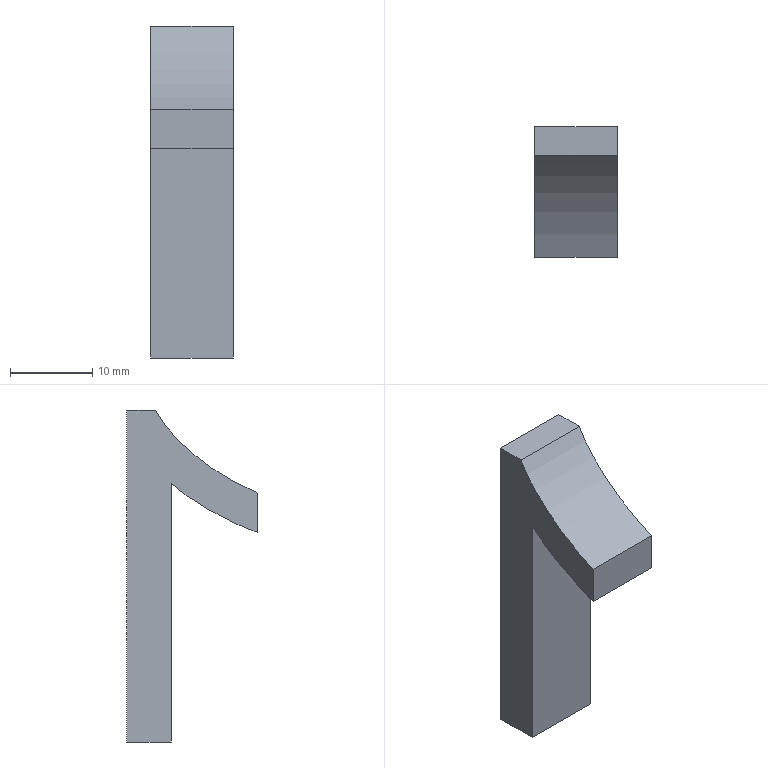Part | NX | features solid 2 | 1 solid | 9 faces | box 10 x 15.893 x 40.382 mm | volume 2722 mm3 | plane 7 | spline 2
STEP:
#1=CARTESIAN_POINT('',(2250.,-427.707,-549.618));
#2=VERTEX_POINT('',#1);
#3=CARTESIAN_POINT('',(2250.,-427.707,-590.));
#4=VERTEX_POINT('',#3);
#5=CARTESIAN_POINT('',(2250.,-427.707,-549.618));
#6=CARTESIAN_POINT('',(2250.,-427.707,-563.078));
#7=CARTESIAN_POINT('',(2250.,-427.707,-576.539));
#8=CARTESIAN_POINT('',(2250.,-427.707,-590.));
#9=B_SPLINE_CURVE_WITH_KNOTS('',3,(#5,#6,#7,#8),.UNSPECIFIED.,.F.,.F.,(4,4),(0.,0.3484),.PIECEWISE_BEZIER_KNOTS.);
#10=EDGE_CURVE('',#2,#4,#9,.T.);
#11=ORIENTED_EDGE('',*,*,#10,.F.);
#12=CARTESIAN_POINT('',(2260.,-427.707,-549.618));
#13=VERTEX_POINT('',#12);
#14=CARTESIAN_POINT('',(2260.,-427.707,-549.618));
#15=DIRECTION('',(-1.,0.,0.));
#16=VECTOR('',#15,1000.);
#17=LINE('',#14,#16);
#18=EDGE_CURVE('',#13,#2,#17,.T.);
#19=ORIENTED_EDGE('',*,*,#18,.F.);
#20=CARTESIAN_POINT('',(2260.,-427.707,-590.));
#21=VERTEX_POINT('',#20);
#22=CARTESIAN_POINT('',(2260.,-427.707,-549.618));
#23=CARTESIAN_POINT('',(2260.,-427.707,-563.078));
#24=CARTESIAN_POINT('',(2260.,-427.707,-576.539));
#25=CARTESIAN_POINT('',(2260.,-427.707,-590.));
#26=B_SPLINE_CURVE_WITH_KNOTS('',3,(#22,#23,#24,#25),.UNSPECIFIED.,.F.,.F.,(4,4),(0.,0.3484),.PIECEWISE_BEZIER_KNOTS.);
#27=EDGE_CURVE('',#13,#21,#26,.T.);
#28=ORIENTED_EDGE('',*,*,#27,.T.);
#29=CARTESIAN_POINT('',(2260.,-427.707,-590.));
#30=DIRECTION('',(-1.,0.,0.));
#31=VECTOR('',#30,1000.);
#32=LINE('',#29,#31);
#33=EDGE_CURVE('',#21,#4,#32,.T.);
#34=ORIENTED_EDGE('',*,*,#33,.T.);
#35=EDGE_LOOP('',(#11,#19,#28,#34));
#36=FACE_BOUND('',#35,.T.);
#37=CARTESIAN_POINT('',(2260.,-427.707,-549.618));
#38=DIRECTION('',(0.,1.,0.));
#39=DIRECTION('',(-1.,0.,0.));
#40=AXIS2_PLACEMENT_3D('',#37,#38,#39);
#41=PLANE('',#40);
#42=ADVANCED_FACE('',(#36),#41,.T.);
#43=CARTESIAN_POINT('',(2250.,-433.137,-590.));
#44=VERTEX_POINT('',#43);
#45=CARTESIAN_POINT('',(2250.,-427.707,-590.));
#46=CARTESIAN_POINT('',(2250.,-429.517,-590.));
#47=CARTESIAN_POINT('',(2250.,-431.327,-590.));
#48=CARTESIAN_POINT('',(2250.,-433.137,-590.));
#49=B_SPLINE_CURVE_WITH_KNOTS('',3,(#45,#46,#47,#48),.UNSPECIFIED.,.F.,.F.,(4,4),(0.3484,0.3952),.PIECEWISE_BEZIER_KNOTS.);
#50=EDGE_CURVE('',#4,#44,#49,.T.);
#51=ORIENTED_EDGE('',*,*,#50,.F.);
#52=ORIENTED_EDGE('',*,*,#33,.F.);
#53=CARTESIAN_POINT('',(2260.,-433.137,-590.));
#54=VERTEX_POINT('',#53);
#55=CARTESIAN_POINT('',(2260.,-427.707,-590.));
#56=CARTESIAN_POINT('',(2260.,-429.517,-590.));
#57=CARTESIAN_POINT('',(2260.,-431.327,-590.));
#58=CARTESIAN_POINT('',(2260.,-433.137,-590.));
#59=B_SPLINE_CURVE_WITH_KNOTS('',3,(#55,#56,#57,#58),.UNSPECIFIED.,.F.,.F.,(4,4),(0.3484,0.3952),.PIECEWISE_BEZIER_KNOTS.);
#60=EDGE_CURVE('',#21,#54,#59,.T.);
#61=ORIENTED_EDGE('',*,*,#60,.T.);
#62=CARTESIAN_POINT('',(2260.,-433.137,-590.));
#63=DIRECTION('',(-1.,0.,0.));
#64=VECTOR('',#63,1000.);
#65=LINE('',#62,#64);
#66=EDGE_CURVE('',#54,#44,#65,.T.);
#67=ORIENTED_EDGE('',*,*,#66,.T.);
#68=EDGE_LOOP('',(#51,#52,#61,#67));
#69=FACE_BOUND('',#68,.T.);
#70=CARTESIAN_POINT('',(2260.,-427.707,-590.));
#71=DIRECTION('',(0.,0.,-1.));
#72=DIRECTION('',(-1.,0.,0.));
#73=AXIS2_PLACEMENT_3D('',#70,#71,#72);
#74=PLANE('',#73);
#75=ADVANCED_FACE('',(#69),#74,.T.);
#76=CARTESIAN_POINT('',(2250.,-433.137,-558.551));
#77=VERTEX_POINT('',#76);
#78=CARTESIAN_POINT('',(2250.,-433.137,-590.));
#79=CARTESIAN_POINT('',(2250.,-433.137,-579.517));
#80=CARTESIAN_POINT('',(2250.,-433.137,-569.034));
#81=CARTESIAN_POINT('',(2250.,-433.137,-558.551));
#82=B_SPLINE_CURVE_WITH_KNOTS('',3,(#78,#79,#80,#81),.UNSPECIFIED.,.F.,.F.,(4,4),(0.3952,0.6666),.PIECEWISE_BEZIER_KNOTS.);
#83=EDGE_CURVE('',#44,#77,#82,.T.);
#84=ORIENTED_EDGE('',*,*,#83,.F.);
#85=ORIENTED_EDGE('',*,*,#66,.F.);
#86=CARTESIAN_POINT('',(2260.,-433.137,-558.551));
#87=VERTEX_POINT('',#86);
#88=CARTESIAN_POINT('',(2260.,-433.137,-590.));
#89=CARTESIAN_POINT('',(2260.,-433.137,-579.517));
#90=CARTESIAN_POINT('',(2260.,-433.137,-569.034));
#91=CARTESIAN_POINT('',(2260.,-433.137,-558.551));
#92=B_SPLINE_CURVE_WITH_KNOTS('',3,(#88,#89,#90,#91),.UNSPECIFIED.,.F.,.F.,(4,4),(0.3952,0.6666),.PIECEWISE_BEZIER_KNOTS.);
#93=EDGE_CURVE('',#54,#87,#92,.T.);
#94=ORIENTED_EDGE('',*,*,#93,.T.);
#95=CARTESIAN_POINT('',(2260.,-433.137,-558.551));
#96=DIRECTION('',(-1.,0.,0.));
#97=VECTOR('',#96,1000.);
#98=LINE('',#95,#97);
#99=EDGE_CURVE('',#87,#77,#98,.T.);
#100=ORIENTED_EDGE('',*,*,#99,.T.);
#101=EDGE_LOOP('',(#84,#85,#94,#100));
#102=FACE_BOUND('',#101,.T.);
#103=CARTESIAN_POINT('',(2260.,-433.137,-590.));
#104=DIRECTION('',(0.,-1.,0.));
#105=DIRECTION('',(1.,0.,0.));
#106=AXIS2_PLACEMENT_3D('',#103,#104,#105);
#107=PLANE('',#106);
#108=ADVANCED_FACE('',(#102),#107,.T.);
#109=CARTESIAN_POINT('',(2250.,-443.6,-564.501));
#110=VERTEX_POINT('',#109);
#111=CARTESIAN_POINT('',(2250.,-433.137,-558.551));
#112=CARTESIAN_POINT('',(2250.,-434.392,-559.713));
#113=CARTESIAN_POINT('',(2250.,-436.074,-560.86));
#114=CARTESIAN_POINT('',(2250.,-440.15,-563.097));
#115=CARTESIAN_POINT('',(2250.,-441.979,-563.966));
#116=CARTESIAN_POINT('',(2250.,-443.6,-564.501));
#117=B_SPLINE_CURVE_WITH_KNOTS('',3,(#111,#112,#113,#114,#115,#116),.UNSPECIFIED.,.F.,.F.,(4,2,4),(0.6666,0.7188,0.7712),.UNSPECIFIED.);
#118=EDGE_CURVE('',#77,#110,#117,.T.);
#119=ORIENTED_EDGE('',*,*,#118,.F.);
#120=ORIENTED_EDGE('',*,*,#99,.F.);
#121=CARTESIAN_POINT('',(2260.,-443.6,-564.501));
#122=VERTEX_POINT('',#121);
#123=CARTESIAN_POINT('',(2260.,-433.137,-558.551));
#124=CARTESIAN_POINT('',(2260.,-434.392,-559.713));
#125=CARTESIAN_POINT('',(2260.,-436.074,-560.86));
#126=CARTESIAN_POINT('',(2260.,-440.15,-563.097));
#127=CARTESIAN_POINT('',(2260.,-441.979,-563.966));
#128=CARTESIAN_POINT('',(2260.,-443.6,-564.501));
#129=B_SPLINE_CURVE_WITH_KNOTS('',3,(#123,#124,#125,#126,#127,#128),.UNSPECIFIED.,.F.,.F.,(4,2,4),(0.6666,0.7188,0.7712),.UNSPECIFIED.);
#130=EDGE_CURVE('',#87,#122,#129,.T.);
#131=ORIENTED_EDGE('',*,*,#130,.T.);
#132=CARTESIAN_POINT('',(2260.,-443.6,-564.501));
#133=DIRECTION('',(-1.,0.,0.));
#134=VECTOR('',#133,1000.);
#135=LINE('',#132,#134);
#136=EDGE_CURVE('',#122,#110,#135,.T.);
#137=ORIENTED_EDGE('',*,*,#136,.T.);
#138=EDGE_LOOP('',(#119,#120,#131,#137));
#139=FACE_BOUND('',#138,.T.);
#140=CARTESIAN_POINT('',(2260.,-433.137,-558.551));
#141=CARTESIAN_POINT('',(2250.,-433.137,-558.551));
#142=CARTESIAN_POINT('',(2260.,-433.765,-559.133));
#143=CARTESIAN_POINT('',(2250.,-433.765,-559.133));
#144=CARTESIAN_POINT('',(2260.,-435.216,-560.282));
#145=CARTESIAN_POINT('',(2250.,-435.216,-560.282));
#146=CARTESIAN_POINT('',(2260.,-438.101,-562.018));
#147=CARTESIAN_POINT('',(2250.,-438.101,-562.018));
#148=CARTESIAN_POINT('',(2260.,-441.088,-563.541));
#149=CARTESIAN_POINT('',(2250.,-441.088,-563.541));
#150=CARTESIAN_POINT('',(2260.,-442.791,-564.234));
#151=CARTESIAN_POINT('',(2250.,-442.791,-564.234));
#152=CARTESIAN_POINT('',(2260.,-443.6,-564.501));
#153=CARTESIAN_POINT('',(2250.,-443.6,-564.501));
#154=B_SPLINE_SURFACE_WITH_KNOTS('',3,1,((#140,#141),(#142,#143),(#144,#145),(#146,#147),(#148,#149),(#150,#151),(#152,#153)),.SURF_OF_LINEAR_EXTRUSION.,.F.,.F.,.F.,(4,1,1,1,4),(2,2),(0.6666,0.6927,0.7189,0.745,0.7712),(0.,1.),.UNSPECIFIED.);
#155=ADVANCED_FACE('',(#139),#154,.T.);
#156=CARTESIAN_POINT('',(2250.,-443.6,-559.713));
#157=VERTEX_POINT('',#156);
#158=CARTESIAN_POINT('',(2250.,-443.6,-564.501));
#159=CARTESIAN_POINT('',(2250.,-443.6,-562.905));
#160=CARTESIAN_POINT('',(2250.,-443.6,-561.309));
#161=CARTESIAN_POINT('',(2250.,-443.6,-559.713));
#162=B_SPLINE_CURVE_WITH_KNOTS('',3,(#158,#159,#160,#161),.UNSPECIFIED.,.F.,.F.,(4,4),(0.7712,0.8125),.PIECEWISE_BEZIER_KNOTS.);
#163=EDGE_CURVE('',#110,#157,#162,.T.);
#164=ORIENTED_EDGE('',*,*,#163,.F.);
#165=ORIENTED_EDGE('',*,*,#136,.F.);
#166=CARTESIAN_POINT('',(2260.,-443.6,-559.713));
#167=VERTEX_POINT('',#166);
#168=CARTESIAN_POINT('',(2260.,-443.6,-564.501));
#169=CARTESIAN_POINT('',(2260.,-443.6,-562.905));
#170=CARTESIAN_POINT('',(2260.,-443.6,-561.309));
#171=CARTESIAN_POINT('',(2260.,-443.6,-559.713));
#172=B_SPLINE_CURVE_WITH_KNOTS('',3,(#168,#169,#170,#171),.UNSPECIFIED.,.F.,.F.,(4,4),(0.7712,0.8125),.PIECEWISE_BEZIER_KNOTS.);
#173=EDGE_CURVE('',#122,#167,#172,.T.);
#174=ORIENTED_EDGE('',*,*,#173,.T.);
#175=CARTESIAN_POINT('',(2260.,-443.6,-559.713));
#176=DIRECTION('',(-1.,0.,0.));
#177=VECTOR('',#176,1000.);
#178=LINE('',#175,#177);
#179=EDGE_CURVE('',#167,#157,#178,.T.);
#180=ORIENTED_EDGE('',*,*,#179,.T.);
#181=EDGE_LOOP('',(#164,#165,#174,#180));
#182=FACE_BOUND('',#181,.T.);
#183=CARTESIAN_POINT('',(2260.,-443.6,-564.501));
#184=DIRECTION('',(0.,-1.,0.));
#185=DIRECTION('',(1.,0.,0.));
#186=AXIS2_PLACEMENT_3D('',#183,#184,#185);
#187=PLANE('',#186);
#188=ADVANCED_FACE('',(#182),#187,.T.);
#189=CARTESIAN_POINT('',(2250.,-431.21,-549.618));
#190=VERTEX_POINT('',#189);
#191=CARTESIAN_POINT('',(2250.,-443.6,-559.713));
#192=CARTESIAN_POINT('',(2250.,-440.678,-558.444));
#193=CARTESIAN_POINT('',(2250.,-438.078,-556.868));
#194=CARTESIAN_POINT('',(2250.,-433.687,-553.183));
#195=CARTESIAN_POINT('',(2250.,-432.128,-551.392));
#196=CARTESIAN_POINT('',(2250.,-431.21,-549.618));
#197=B_SPLINE_CURVE_WITH_KNOTS('',3,(#191,#192,#193,#194,#195,#196),.UNSPECIFIED.,.F.,.F.,(4,2,4),(0.8125,0.8906,0.9692),.UNSPECIFIED.);
#198=EDGE_CURVE('',#157,#190,#197,.T.);
#199=ORIENTED_EDGE('',*,*,#198,.F.);
#200=ORIENTED_EDGE('',*,*,#179,.F.);
#201=CARTESIAN_POINT('',(2260.,-431.21,-549.618));
#202=VERTEX_POINT('',#201);
#203=CARTESIAN_POINT('',(2260.,-443.6,-559.713));
#204=CARTESIAN_POINT('',(2260.,-440.678,-558.444));
#205=CARTESIAN_POINT('',(2260.,-438.078,-556.868));
#206=CARTESIAN_POINT('',(2260.,-433.687,-553.183));
#207=CARTESIAN_POINT('',(2260.,-432.128,-551.392));
#208=CARTESIAN_POINT('',(2260.,-431.21,-549.618));
#209=B_SPLINE_CURVE_WITH_KNOTS('',3,(#203,#204,#205,#206,#207,#208),.UNSPECIFIED.,.F.,.F.,(4,2,4),(0.8125,0.8906,0.9692),.UNSPECIFIED.);
#210=EDGE_CURVE('',#167,#202,#209,.T.);
#211=ORIENTED_EDGE('',*,*,#210,.T.);
#212=CARTESIAN_POINT('',(2260.,-431.21,-549.618));
#213=DIRECTION('',(-1.,0.,0.));
#214=VECTOR('',#213,1000.);
#215=LINE('',#212,#214);
#216=EDGE_CURVE('',#202,#190,#215,.T.);
#217=ORIENTED_EDGE('',*,*,#216,.T.);
#218=EDGE_LOOP('',(#199,#200,#211,#217));
#219=FACE_BOUND('',#218,.T.);
#220=CARTESIAN_POINT('',(2260.,-443.6,-559.713));
#221=CARTESIAN_POINT('',(2250.,-443.6,-559.713));
#222=CARTESIAN_POINT('',(2260.,-442.134,-559.076));
#223=CARTESIAN_POINT('',(2250.,-442.134,-559.076));
#224=CARTESIAN_POINT('',(2260.,-439.371,-557.659));
#225=CARTESIAN_POINT('',(2250.,-439.371,-557.659));
#226=CARTESIAN_POINT('',(2260.,-435.733,-555.036));
#227=CARTESIAN_POINT('',(2250.,-435.733,-555.036));
#228=CARTESIAN_POINT('',(2260.,-432.892,-552.266));
#229=CARTESIAN_POINT('',(2250.,-432.892,-552.266));
#230=CARTESIAN_POINT('',(2260.,-431.667,-550.501));
#231=CARTESIAN_POINT('',(2250.,-431.667,-550.501));
#232=CARTESIAN_POINT('',(2260.,-431.21,-549.618));
#233=CARTESIAN_POINT('',(2250.,-431.21,-549.618));
#234=B_SPLINE_SURFACE_WITH_KNOTS('',3,1,((#220,#221),(#222,#223),(#224,#225),(#226,#227),(#228,#229),(#230,#231),(#232,#233)),.SURF_OF_LINEAR_EXTRUSION.,.F.,.F.,.F.,(4,1,1,1,4),(2,2),(0.8125,0.8517,0.8909,0.9301,0.9692),(0.,1.),.UNSPECIFIED.);
#235=ADVANCED_FACE('',(#219),#234,.T.);
#236=CARTESIAN_POINT('',(2250.,-431.21,-549.618));
#237=CARTESIAN_POINT('',(2250.,-430.042,-549.618));
#238=CARTESIAN_POINT('',(2250.,-428.875,-549.618));
#239=CARTESIAN_POINT('',(2250.,-427.707,-549.618));
#240=B_SPLINE_CURVE_WITH_KNOTS('',3,(#236,#237,#238,#239),.UNSPECIFIED.,.F.,.F.,(4,4),(0.9692,1.),.PIECEWISE_BEZIER_KNOTS.);
#241=EDGE_CURVE('',#190,#2,#240,.T.);
#242=ORIENTED_EDGE('',*,*,#241,.F.);
#243=ORIENTED_EDGE('',*,*,#216,.F.);
#244=CARTESIAN_POINT('',(2260.,-431.21,-549.618));
#245=CARTESIAN_POINT('',(2260.,-430.042,-549.618));
#246=CARTESIAN_POINT('',(2260.,-428.875,-549.618));
#247=CARTESIAN_POINT('',(2260.,-427.707,-549.618));
#248=B_SPLINE_CURVE_WITH_KNOTS('',3,(#244,#245,#246,#247),.UNSPECIFIED.,.F.,.F.,(4,4),(0.9692,1.),.PIECEWISE_BEZIER_KNOTS.);
#249=EDGE_CURVE('',#202,#13,#248,.T.);
#250=ORIENTED_EDGE('',*,*,#249,.T.);
#251=ORIENTED_EDGE('',*,*,#18,.T.);
#252=EDGE_LOOP('',(#242,#243,#250,#251));
#253=FACE_BOUND('',#252,.T.);
#254=CARTESIAN_POINT('',(2260.,-431.21,-549.618));
#255=DIRECTION('',(0.,0.,1.));
#256=DIRECTION('',(0.,-1.,0.));
#257=AXIS2_PLACEMENT_3D('',#254,#255,#256);
#258=PLANE('',#257);
#259=ADVANCED_FACE('',(#253),#258,.T.);
#260=ORIENTED_EDGE('',*,*,#27,.F.);
#261=ORIENTED_EDGE('',*,*,#249,.F.);
#262=ORIENTED_EDGE('',*,*,#210,.F.);
#263=ORIENTED_EDGE('',*,*,#173,.F.);
#264=ORIENTED_EDGE('',*,*,#130,.F.);
#265=ORIENTED_EDGE('',*,*,#93,.F.);
#266=ORIENTED_EDGE('',*,*,#60,.F.);
#267=EDGE_LOOP('',(#260,#261,#262,#263,#264,#265,#266));
#268=FACE_BOUND('',#267,.T.);
#269=CARTESIAN_POINT('',(2260.,-438.118,-561.982));
#270=DIRECTION('',(1.,0.,0.));
#271=DIRECTION('',(0.,1.,0.));
#272=AXIS2_PLACEMENT_3D('',#269,#270,#271);
#273=PLANE('',#272);
#274=ADVANCED_FACE('',(#268),#273,.T.);
#275=ORIENTED_EDGE('',*,*,#10,.T.);
#276=ORIENTED_EDGE('',*,*,#50,.T.);
#277=ORIENTED_EDGE('',*,*,#83,.T.);
#278=ORIENTED_EDGE('',*,*,#118,.T.);
#279=ORIENTED_EDGE('',*,*,#163,.T.);
#280=ORIENTED_EDGE('',*,*,#198,.T.);
#281=ORIENTED_EDGE('',*,*,#241,.T.);
#282=EDGE_LOOP('',(#275,#276,#277,#278,#279,#280,#281));
#283=FACE_BOUND('',#282,.T.);
#284=CARTESIAN_POINT('',(2250.,-438.118,-561.982));
#285=DIRECTION('',(1.,0.,0.));
#286=DIRECTION('',(0.,1.,0.));
#287=AXIS2_PLACEMENT_3D('',#284,#285,#286);
#288=PLANE('',#287);
#289=ADVANCED_FACE('',(#283),#288,.F.);
#290=CLOSED_SHELL('',(#42,#75,#108,#155,#188,#235,#259,#274,#289));
#291=MANIFOLD_SOLID_BREP('',#290);
#292=(LENGTH_UNIT()NAMED_UNIT(*)SI_UNIT(.MILLI.,.METRE.));
#293=UNCERTAINTY_MEASURE_WITH_UNIT(LENGTH_MEASURE(0.0508),#292,'','');
#294=(NAMED_UNIT(*)PLANE_ANGLE_UNIT()SI_UNIT($,.RADIAN.));
#295=(NAMED_UNIT(*)SI_UNIT($,.STERADIAN.)SOLID_ANGLE_UNIT());
#296=(GEOMETRIC_REPRESENTATION_CONTEXT(3)GLOBAL_UNCERTAINTY_ASSIGNED_CONTEXT((#293))GLOBAL_UNIT_ASSIGNED_CONTEXT((#292,#294,#295))REPRESENTATION_CONTEXT('',''));
#297=ADVANCED_BREP_SHAPE_REPRESENTATION('',(#291),#296);